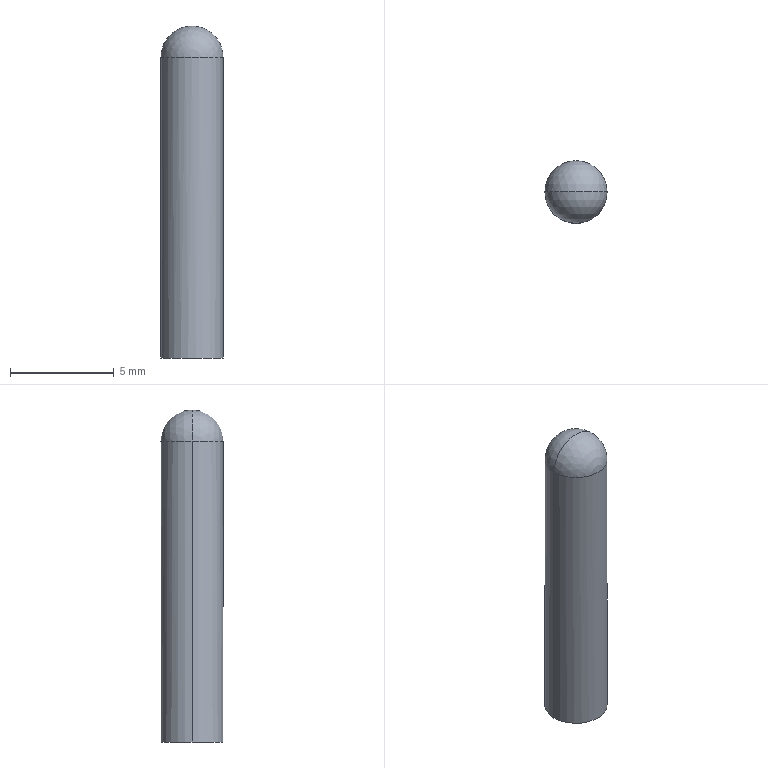Part | SolidWorks | features Extrusion 1, Fillet 1 | 1 solid | 5 faces | box 3 x 3 x 16 mm | volume 109.563 mm3 | sphere 2 | cylinder 2 | plane 1 | commonest cylinder face diameters 3 x2
STEP:
#1=CARTESIAN_POINT('',(-1.5,0.,14.5));
#2=VERTEX_POINT('',#1);
#3=CARTESIAN_POINT('',(1.5,0.,14.5));
#4=VERTEX_POINT('',#3);
#5=CARTESIAN_POINT('',(0.,0.,14.5));
#6=DIRECTION('',(0.,0.,-1.));
#7=DIRECTION('',(-1.,0.,0.));
#8=AXIS2_PLACEMENT_3D('',#5,#6,#7);
#9=CIRCLE('',#8,1.5);
#10=EDGE_CURVE('',#2,#4,#9,.T.);
#11=ORIENTED_EDGE('',*,*,#10,.F.);
#12=CARTESIAN_POINT('',(0.,0.,16.));
#13=VERTEX_POINT('',#12);
#14=CARTESIAN_POINT('',(0.,0.,14.5));
#15=DIRECTION('',(0.,1.,0.));
#16=DIRECTION('',(-1.,0.,0.));
#17=AXIS2_PLACEMENT_3D('',#14,#15,#16);
#18=CIRCLE('',#17,1.5);
#19=EDGE_CURVE('',#2,#13,#18,.T.);
#20=ORIENTED_EDGE('',*,*,#19,.T.);
#21=CARTESIAN_POINT('',(0.,0.,14.5));
#22=DIRECTION('',(0.,-1.,0.));
#23=DIRECTION('',(0.,0.,-1.));
#24=AXIS2_PLACEMENT_3D('',#21,#22,#23);
#25=CIRCLE('',#24,1.5);
#26=EDGE_CURVE('',#4,#13,#25,.T.);
#27=ORIENTED_EDGE('',*,*,#26,.F.);
#28=EDGE_LOOP('',(#11,#20,#27));
#29=FACE_OUTER_BOUND('',#28,.T.);
#30=CARTESIAN_POINT('',(0.,0.,14.5));
#31=DIRECTION('',(0.,1.,0.));
#32=DIRECTION('',(1.,0.,0.));
#33=AXIS2_PLACEMENT_3D('',#30,#31,#32);
#34=SPHERICAL_SURFACE('',#33,1.5);
#35=ADVANCED_FACE('',(#29),#34,.T.);
#36=ORIENTED_EDGE('',*,*,#10,.T.);
#37=CARTESIAN_POINT('',(1.5,0.,0.));
#38=VERTEX_POINT('',#37);
#39=CARTESIAN_POINT('',(1.5,0.,16.));
#40=DIRECTION('',(0.,0.,-1.));
#41=VECTOR('',#40,1000.);
#42=LINE('',#39,#41);
#43=EDGE_CURVE('',#4,#38,#42,.T.);
#44=ORIENTED_EDGE('',*,*,#43,.T.);
#45=CARTESIAN_POINT('',(-1.5,0.,0.));
#46=VERTEX_POINT('',#45);
#47=CARTESIAN_POINT('',(0.,0.,0.));
#48=DIRECTION('',(0.,0.,1.));
#49=DIRECTION('',(1.,0.,0.));
#50=AXIS2_PLACEMENT_3D('',#47,#48,#49);
#51=CIRCLE('',#50,1.5);
#52=EDGE_CURVE('',#38,#46,#51,.T.);
#53=ORIENTED_EDGE('',*,*,#52,.T.);
#54=CARTESIAN_POINT('',(-1.5,0.,16.));
#55=DIRECTION('',(0.,0.,-1.));
#56=VECTOR('',#55,1000.);
#57=LINE('',#54,#56);
#58=EDGE_CURVE('',#2,#46,#57,.T.);
#59=ORIENTED_EDGE('',*,*,#58,.F.);
#60=EDGE_LOOP('',(#36,#44,#53,#59));
#61=FACE_OUTER_BOUND('',#60,.T.);
#62=CARTESIAN_POINT('',(0.,0.,16.));
#63=DIRECTION('',(0.,0.,-1.));
#64=DIRECTION('',(-1.,0.,0.));
#65=AXIS2_PLACEMENT_3D('',#62,#63,#64);
#66=CYLINDRICAL_SURFACE('',#65,1.5);
#67=ADVANCED_FACE('',(#61),#66,.T.);
#68=ORIENTED_EDGE('',*,*,#43,.F.);
#69=CARTESIAN_POINT('',(0.,0.,14.5));
#70=DIRECTION('',(0.,0.,-1.));
#71=DIRECTION('',(-1.,0.,0.));
#72=AXIS2_PLACEMENT_3D('',#69,#70,#71);
#73=CIRCLE('',#72,1.5);
#74=EDGE_CURVE('',#4,#2,#73,.T.);
#75=ORIENTED_EDGE('',*,*,#74,.T.);
#76=ORIENTED_EDGE('',*,*,#58,.T.);
#77=CARTESIAN_POINT('',(0.,0.,0.));
#78=DIRECTION('',(0.,0.,1.));
#79=DIRECTION('',(1.,0.,0.));
#80=AXIS2_PLACEMENT_3D('',#77,#78,#79);
#81=CIRCLE('',#80,1.5);
#82=EDGE_CURVE('',#46,#38,#81,.T.);
#83=ORIENTED_EDGE('',*,*,#82,.T.);
#84=EDGE_LOOP('',(#68,#75,#76,#83));
#85=FACE_OUTER_BOUND('',#84,.T.);
#86=CARTESIAN_POINT('',(0.,0.,16.));
#87=DIRECTION('',(0.,0.,-1.));
#88=DIRECTION('',(-1.,0.,0.));
#89=AXIS2_PLACEMENT_3D('',#86,#87,#88);
#90=CYLINDRICAL_SURFACE('',#89,1.5);
#91=ADVANCED_FACE('',(#85),#90,.T.);
#92=ORIENTED_EDGE('',*,*,#82,.F.);
#93=ORIENTED_EDGE('',*,*,#52,.F.);
#94=EDGE_LOOP('',(#92,#93));
#95=FACE_OUTER_BOUND('',#94,.T.);
#96=CARTESIAN_POINT('',(0.,0.,0.));
#97=DIRECTION('',(0.,0.,1.));
#98=DIRECTION('',(1.,0.,0.));
#99=AXIS2_PLACEMENT_3D('',#96,#97,#98);
#100=PLANE('',#99);
#101=ADVANCED_FACE('',(#95),#100,.F.);
#102=ORIENTED_EDGE('',*,*,#19,.F.);
#103=ORIENTED_EDGE('',*,*,#74,.F.);
#104=ORIENTED_EDGE('',*,*,#26,.T.);
#105=EDGE_LOOP('',(#102,#103,#104));
#106=FACE_OUTER_BOUND('',#105,.T.);
#107=CARTESIAN_POINT('',(0.,0.,14.5));
#108=DIRECTION('',(0.,1.,0.));
#109=DIRECTION('',(1.,0.,0.));
#110=AXIS2_PLACEMENT_3D('',#107,#108,#109);
#111=SPHERICAL_SURFACE('',#110,1.5);
#112=ADVANCED_FACE('',(#106),#111,.T.);
#113=CLOSED_SHELL('',(#35,#67,#91,#101,#112));
#114=MANIFOLD_SOLID_BREP('',#113);
#115=CARTESIAN_POINT('',(0.,0.,0.));
#116=DIRECTION('',(0.,0.,1.));
#117=DIRECTION('',(1.,0.,0.));
#118=AXIS2_PLACEMENT_3D('',#115,#116,#117);
#119=(LENGTH_UNIT()NAMED_UNIT(*)SI_UNIT(.MILLI.,.METRE.));
#120=UNCERTAINTY_MEASURE_WITH_UNIT(LENGTH_MEASURE(0.00001),#119,'','');
#121=(NAMED_UNIT(*)PLANE_ANGLE_UNIT()SI_UNIT($,.RADIAN.));
#122=(NAMED_UNIT(*)SI_UNIT($,.STERADIAN.)SOLID_ANGLE_UNIT());
#123=(GEOMETRIC_REPRESENTATION_CONTEXT(3)GLOBAL_UNCERTAINTY_ASSIGNED_CONTEXT((#120))GLOBAL_UNIT_ASSIGNED_CONTEXT((#119,#121,#122))REPRESENTATION_CONTEXT('',''));
#124=ADVANCED_BREP_SHAPE_REPRESENTATION('',(#114,#118),#123);